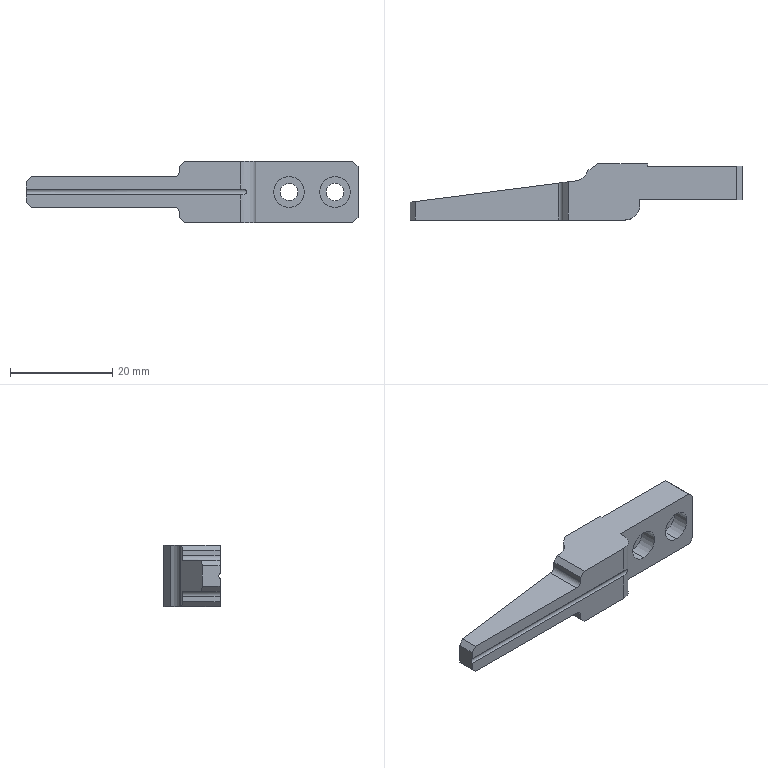Part | SolidWorks | features ICE 5, Chamfer 4, Fillet 2, Extrusion 1, HoleWzd 1 | 1 solid | 38 faces | box 65 x 11 x 12 mm | volume 4036 mm3 | plane 25 | cylinder 13 | commonest cylinder face diameters 6 x6 3.4 x4 2 x2 1.5 x1
STEP:
#1=CARTESIAN_POINT('',(28.,7.4,3.));
#2=VERTEX_POINT('',#1);
#3=CARTESIAN_POINT('',(28.,7.4,-3.));
#4=VERTEX_POINT('',#3);
#5=CARTESIAN_POINT('',(28.,7.4,0.));
#6=DIRECTION('',(0.,-1.,0.));
#7=DIRECTION('',(0.,0.,-1.));
#8=AXIS2_PLACEMENT_3D('',#5,#6,#7);
#9=CIRCLE('',#8,3.);
#10=EDGE_CURVE('',#2,#4,#9,.T.);
#11=ORIENTED_EDGE('',*,*,#10,.F.);
#12=CARTESIAN_POINT('',(28.,4.,3.));
#13=VERTEX_POINT('',#12);
#14=CARTESIAN_POINT('',(28.,4.,3.));
#15=DIRECTION('',(0.,-1.,0.));
#16=VECTOR('',#15,1000.);
#17=LINE('',#14,#16);
#18=EDGE_CURVE('',#2,#13,#17,.T.);
#19=ORIENTED_EDGE('',*,*,#18,.T.);
#20=CARTESIAN_POINT('',(28.,4.,-3.));
#21=VERTEX_POINT('',#20);
#22=CARTESIAN_POINT('',(28.,4.,0.));
#23=DIRECTION('',(0.,-1.,0.));
#24=DIRECTION('',(0.,0.,-1.));
#25=AXIS2_PLACEMENT_3D('',#22,#23,#24);
#26=CIRCLE('',#25,3.);
#27=EDGE_CURVE('',#13,#21,#26,.T.);
#28=ORIENTED_EDGE('',*,*,#27,.T.);
#29=CARTESIAN_POINT('',(28.,4.,-3.));
#30=DIRECTION('',(0.,-1.,0.));
#31=VECTOR('',#30,1000.);
#32=LINE('',#29,#31);
#33=EDGE_CURVE('',#4,#21,#32,.T.);
#34=ORIENTED_EDGE('',*,*,#33,.F.);
#35=EDGE_LOOP('',(#11,#19,#28,#34));
#36=FACE_OUTER_BOUND('',#35,.T.);
#37=CARTESIAN_POINT('',(28.,4.,0.));
#38=DIRECTION('',(0.,-1.,0.));
#39=DIRECTION('',(0.,0.,-1.));
#40=AXIS2_PLACEMENT_3D('',#37,#38,#39);
#41=CYLINDRICAL_SURFACE('',#40,3.);
#42=ADVANCED_FACE('',(#36),#41,.F.);
#43=CARTESIAN_POINT('',(19.,7.4,3.));
#44=VERTEX_POINT('',#43);
#45=CARTESIAN_POINT('',(19.,7.4,-3.));
#46=VERTEX_POINT('',#45);
#47=CARTESIAN_POINT('',(19.,7.4,0.));
#48=DIRECTION('',(0.,-1.,0.));
#49=DIRECTION('',(0.,0.,-1.));
#50=AXIS2_PLACEMENT_3D('',#47,#48,#49);
#51=CIRCLE('',#50,3.);
#52=EDGE_CURVE('',#44,#46,#51,.T.);
#53=ORIENTED_EDGE('',*,*,#52,.F.);
#54=CARTESIAN_POINT('',(19.,4.,3.));
#55=VERTEX_POINT('',#54);
#56=CARTESIAN_POINT('',(19.,4.,3.));
#57=DIRECTION('',(0.,-1.,0.));
#58=VECTOR('',#57,1000.);
#59=LINE('',#56,#58);
#60=EDGE_CURVE('',#44,#55,#59,.T.);
#61=ORIENTED_EDGE('',*,*,#60,.T.);
#62=CARTESIAN_POINT('',(19.,4.,-3.));
#63=VERTEX_POINT('',#62);
#64=CARTESIAN_POINT('',(19.,4.,0.));
#65=DIRECTION('',(0.,-1.,0.));
#66=DIRECTION('',(0.,0.,-1.));
#67=AXIS2_PLACEMENT_3D('',#64,#65,#66);
#68=CIRCLE('',#67,3.);
#69=EDGE_CURVE('',#55,#63,#68,.T.);
#70=ORIENTED_EDGE('',*,*,#69,.T.);
#71=CARTESIAN_POINT('',(19.,4.,-3.));
#72=DIRECTION('',(0.,-1.,0.));
#73=VECTOR('',#72,1000.);
#74=LINE('',#71,#73);
#75=EDGE_CURVE('',#46,#63,#74,.T.);
#76=ORIENTED_EDGE('',*,*,#75,.F.);
#77=EDGE_LOOP('',(#53,#61,#70,#76));
#78=FACE_OUTER_BOUND('',#77,.T.);
#79=CARTESIAN_POINT('',(19.,4.,0.));
#80=DIRECTION('',(0.,-1.,0.));
#81=DIRECTION('',(0.,0.,-1.));
#82=AXIS2_PLACEMENT_3D('',#79,#80,#81);
#83=CYLINDRICAL_SURFACE('',#82,3.);
#84=ADVANCED_FACE('',(#78),#83,.F.);
#85=CARTESIAN_POINT('',(28.,10.5,1.7));
#86=VERTEX_POINT('',#85);
#87=CARTESIAN_POINT('',(28.,10.5,-1.7));
#88=VERTEX_POINT('',#87);
#89=CARTESIAN_POINT('',(28.,10.5,0.));
#90=DIRECTION('',(0.,-1.,0.));
#91=DIRECTION('',(0.,0.,1.));
#92=AXIS2_PLACEMENT_3D('',#89,#90,#91);
#93=CIRCLE('',#92,1.7);
#94=EDGE_CURVE('',#86,#88,#93,.T.);
#95=ORIENTED_EDGE('',*,*,#94,.F.);
#96=CARTESIAN_POINT('',(28.,7.4,1.7));
#97=VERTEX_POINT('',#96);
#98=CARTESIAN_POINT('',(28.,4.,1.7));
#99=DIRECTION('',(0.,-1.,0.));
#100=VECTOR('',#99,1000.);
#101=LINE('',#98,#100);
#102=EDGE_CURVE('',#86,#97,#101,.T.);
#103=ORIENTED_EDGE('',*,*,#102,.T.);
#104=CARTESIAN_POINT('',(28.,7.4,-1.7));
#105=VERTEX_POINT('',#104);
#106=CARTESIAN_POINT('',(28.,7.4,0.));
#107=DIRECTION('',(0.,-1.,0.));
#108=DIRECTION('',(0.,0.,-1.));
#109=AXIS2_PLACEMENT_3D('',#106,#107,#108);
#110=CIRCLE('',#109,1.7);
#111=EDGE_CURVE('',#97,#105,#110,.T.);
#112=ORIENTED_EDGE('',*,*,#111,.T.);
#113=CARTESIAN_POINT('',(28.,4.,-1.7));
#114=DIRECTION('',(0.,-1.,0.));
#115=VECTOR('',#114,1000.);
#116=LINE('',#113,#115);
#117=EDGE_CURVE('',#88,#105,#116,.T.);
#118=ORIENTED_EDGE('',*,*,#117,.F.);
#119=EDGE_LOOP('',(#95,#103,#112,#118));
#120=FACE_OUTER_BOUND('',#119,.T.);
#121=CARTESIAN_POINT('',(28.,4.,0.));
#122=DIRECTION('',(0.,-1.,0.));
#123=DIRECTION('',(0.,0.,-1.));
#124=AXIS2_PLACEMENT_3D('',#121,#122,#123);
#125=CYLINDRICAL_SURFACE('',#124,1.7);
#126=ADVANCED_FACE('',(#120),#125,.F.);
#127=CARTESIAN_POINT('',(19.,10.5,1.7));
#128=VERTEX_POINT('',#127);
#129=CARTESIAN_POINT('',(19.,10.5,-1.7));
#130=VERTEX_POINT('',#129);
#131=CARTESIAN_POINT('',(19.,10.5,0.));
#132=DIRECTION('',(0.,-1.,0.));
#133=DIRECTION('',(0.,0.,1.));
#134=AXIS2_PLACEMENT_3D('',#131,#132,#133);
#135=CIRCLE('',#134,1.7);
#136=EDGE_CURVE('',#128,#130,#135,.T.);
#137=ORIENTED_EDGE('',*,*,#136,.F.);
#138=CARTESIAN_POINT('',(19.,7.4,1.7));
#139=VERTEX_POINT('',#138);
#140=CARTESIAN_POINT('',(19.,4.,1.7));
#141=DIRECTION('',(0.,-1.,0.));
#142=VECTOR('',#141,1000.);
#143=LINE('',#140,#142);
#144=EDGE_CURVE('',#128,#139,#143,.T.);
#145=ORIENTED_EDGE('',*,*,#144,.T.);
#146=CARTESIAN_POINT('',(19.,7.4,-1.7));
#147=VERTEX_POINT('',#146);
#148=CARTESIAN_POINT('',(19.,7.4,0.));
#149=DIRECTION('',(0.,-1.,0.));
#150=DIRECTION('',(0.,0.,-1.));
#151=AXIS2_PLACEMENT_3D('',#148,#149,#150);
#152=CIRCLE('',#151,1.7);
#153=EDGE_CURVE('',#139,#147,#152,.T.);
#154=ORIENTED_EDGE('',*,*,#153,.T.);
#155=CARTESIAN_POINT('',(19.,4.,-1.7));
#156=DIRECTION('',(0.,-1.,0.));
#157=VECTOR('',#156,1000.);
#158=LINE('',#155,#157);
#159=EDGE_CURVE('',#130,#147,#158,.T.);
#160=ORIENTED_EDGE('',*,*,#159,.F.);
#161=EDGE_LOOP('',(#137,#145,#154,#160));
#162=FACE_OUTER_BOUND('',#161,.T.);
#163=CARTESIAN_POINT('',(19.,4.,0.));
#164=DIRECTION('',(0.,-1.,0.));
#165=DIRECTION('',(0.,0.,-1.));
#166=AXIS2_PLACEMENT_3D('',#163,#164,#165);
#167=CYLINDRICAL_SURFACE('',#166,1.7);
#168=ADVANCED_FACE('',(#162),#167,.F.);
#169=CARTESIAN_POINT('',(32.5,10.5,5.));
#170=VERTEX_POINT('',#169);
#171=CARTESIAN_POINT('',(32.5,10.5,-5.));
#172=VERTEX_POINT('',#171);
#173=CARTESIAN_POINT('',(32.5,10.5,-6.));
#174=DIRECTION('',(0.,0.,-1.));
#175=VECTOR('',#174,1000.);
#176=LINE('',#173,#175);
#177=EDGE_CURVE('',#170,#172,#176,.T.);
#178=ORIENTED_EDGE('',*,*,#177,.F.);
#179=CARTESIAN_POINT('',(32.5,4.,5.));
#180=VERTEX_POINT('',#179);
#181=CARTESIAN_POINT('',(32.5,11.,5.));
#182=DIRECTION('',(0.,-1.,0.));
#183=VECTOR('',#182,1000.);
#184=LINE('',#181,#183);
#185=EDGE_CURVE('',#170,#180,#184,.T.);
#186=ORIENTED_EDGE('',*,*,#185,.T.);
#187=CARTESIAN_POINT('',(32.5,4.,-5.));
#188=VERTEX_POINT('',#187);
#189=CARTESIAN_POINT('',(32.5,4.,-14.));
#190=DIRECTION('',(0.,0.,1.));
#191=VECTOR('',#190,1000.);
#192=LINE('',#189,#191);
#193=EDGE_CURVE('',#188,#180,#192,.T.);
#194=ORIENTED_EDGE('',*,*,#193,.F.);
#195=CARTESIAN_POINT('',(32.5,11.,-5.));
#196=DIRECTION('',(0.,1.,0.));
#197=VECTOR('',#196,1000.);
#198=LINE('',#195,#197);
#199=EDGE_CURVE('',#188,#172,#198,.T.);
#200=ORIENTED_EDGE('',*,*,#199,.T.);
#201=EDGE_LOOP('',(#178,#186,#194,#200));
#202=FACE_OUTER_BOUND('',#201,.T.);
#203=CARTESIAN_POINT('',(32.5,11.,-6.));
#204=DIRECTION('',(-1.,0.,0.));
#205=DIRECTION('',(0.,0.,1.));
#206=AXIS2_PLACEMENT_3D('',#203,#204,#205);
#207=PLANE('',#206);
#208=ADVANCED_FACE('',(#202),#207,.F.);
#209=ORIENTED_EDGE('',*,*,#185,.F.);
#210=CARTESIAN_POINT('',(31.5,10.5,6.));
#211=VERTEX_POINT('',#210);
#212=CARTESIAN_POINT('',(32.5,10.5,5.));
#213=DIRECTION('',(-0.7071,0.,0.7071));
#214=VECTOR('',#213,1000.);
#215=LINE('',#212,#214);
#216=EDGE_CURVE('',#170,#211,#215,.T.);
#217=ORIENTED_EDGE('',*,*,#216,.T.);
#218=CARTESIAN_POINT('',(31.5,4.,6.));
#219=VERTEX_POINT('',#218);
#220=CARTESIAN_POINT('',(31.5,11.,6.));
#221=DIRECTION('',(0.,1.,0.));
#222=VECTOR('',#221,1000.);
#223=LINE('',#220,#222);
#224=EDGE_CURVE('',#219,#211,#223,.T.);
#225=ORIENTED_EDGE('',*,*,#224,.F.);
#226=CARTESIAN_POINT('',(32.5,4.,5.));
#227=DIRECTION('',(-0.7071,0.,0.7071));
#228=VECTOR('',#227,1000.);
#229=LINE('',#226,#228);
#230=EDGE_CURVE('',#180,#219,#229,.T.);
#231=ORIENTED_EDGE('',*,*,#230,.F.);
#232=EDGE_LOOP('',(#209,#217,#225,#231));
#233=FACE_OUTER_BOUND('',#232,.T.);
#234=CARTESIAN_POINT('',(32.5,11.,5.));
#235=DIRECTION('',(-0.7071,0.,-0.7071));
#236=DIRECTION('',(0.,-1.,0.));
#237=AXIS2_PLACEMENT_3D('',#234,#235,#236);
#238=PLANE('',#237);
#239=ADVANCED_FACE('',(#233),#238,.F.);
#240=CARTESIAN_POINT('',(31.5,10.5,-6.));
#241=VERTEX_POINT('',#240);
#242=CARTESIAN_POINT('',(31.5,4.,-6.));
#243=VERTEX_POINT('',#242);
#244=CARTESIAN_POINT('',(31.5,11.,-6.));
#245=DIRECTION('',(0.,-1.,0.));
#246=VECTOR('',#245,1000.);
#247=LINE('',#244,#246);
#248=EDGE_CURVE('',#241,#243,#247,.T.);
#249=ORIENTED_EDGE('',*,*,#248,.F.);
#250=CARTESIAN_POINT('',(31.5,10.5,-6.));
#251=DIRECTION('',(0.7071,0.,0.7071));
#252=VECTOR('',#251,1000.);
#253=LINE('',#250,#252);
#254=EDGE_CURVE('',#241,#172,#253,.T.);
#255=ORIENTED_EDGE('',*,*,#254,.T.);
#256=ORIENTED_EDGE('',*,*,#199,.F.);
#257=CARTESIAN_POINT('',(31.5,4.,-6.));
#258=DIRECTION('',(0.7071,0.,0.7071));
#259=VECTOR('',#258,1000.);
#260=LINE('',#257,#259);
#261=EDGE_CURVE('',#243,#188,#260,.T.);
#262=ORIENTED_EDGE('',*,*,#261,.F.);
#263=EDGE_LOOP('',(#249,#255,#256,#262));
#264=FACE_OUTER_BOUND('',#263,.T.);
#265=CARTESIAN_POINT('',(31.5,11.,-6.));
#266=DIRECTION('',(-0.7071,0.,0.7071));
#267=DIRECTION('',(0.,-1.,0.));
#268=AXIS2_PLACEMENT_3D('',#265,#266,#267);
#269=PLANE('',#268);
#270=ADVANCED_FACE('',(#264),#269,.F.);
#271=ORIENTED_EDGE('',*,*,#144,.F.);
#272=CARTESIAN_POINT('',(19.,10.5,0.));
#273=DIRECTION('',(0.,-1.,0.));
#274=DIRECTION('',(0.,0.,1.));
#275=AXIS2_PLACEMENT_3D('',#272,#273,#274);
#276=CIRCLE('',#275,1.7);
#277=EDGE_CURVE('',#130,#128,#276,.T.);
#278=ORIENTED_EDGE('',*,*,#277,.F.);
#279=ORIENTED_EDGE('',*,*,#159,.T.);
#280=CARTESIAN_POINT('',(19.,7.4,0.));
#281=DIRECTION('',(0.,-1.,0.));
#282=DIRECTION('',(0.,0.,-1.));
#283=AXIS2_PLACEMENT_3D('',#280,#281,#282);
#284=CIRCLE('',#283,1.7);
#285=EDGE_CURVE('',#147,#139,#284,.T.);
#286=ORIENTED_EDGE('',*,*,#285,.T.);
#287=EDGE_LOOP('',(#271,#278,#279,#286));
#288=FACE_OUTER_BOUND('',#287,.T.);
#289=CARTESIAN_POINT('',(19.,4.,0.));
#290=DIRECTION('',(0.,-1.,0.));
#291=DIRECTION('',(0.,0.,-1.));
#292=AXIS2_PLACEMENT_3D('',#289,#290,#291);
#293=CYLINDRICAL_SURFACE('',#292,1.7);
#294=ADVANCED_FACE('',(#288),#293,.F.);
#295=ORIENTED_EDGE('',*,*,#102,.F.);
#296=CARTESIAN_POINT('',(28.,10.5,0.));
#297=DIRECTION('',(0.,-1.,0.));
#298=DIRECTION('',(0.,0.,1.));
#299=AXIS2_PLACEMENT_3D('',#296,#297,#298);
#300=CIRCLE('',#299,1.7);
#301=EDGE_CURVE('',#88,#86,#300,.T.);
#302=ORIENTED_EDGE('',*,*,#301,.F.);
#303=ORIENTED_EDGE('',*,*,#117,.T.);
#304=CARTESIAN_POINT('',(28.,7.4,0.));
#305=DIRECTION('',(0.,-1.,0.));
#306=DIRECTION('',(0.,0.,-1.));
#307=AXIS2_PLACEMENT_3D('',#304,#305,#306);
#308=CIRCLE('',#307,1.7);
#309=EDGE_CURVE('',#105,#97,#308,.T.);
#310=ORIENTED_EDGE('',*,*,#309,.T.);
#311=EDGE_LOOP('',(#295,#302,#303,#310));
#312=FACE_OUTER_BOUND('',#311,.T.);
#313=CARTESIAN_POINT('',(28.,4.,0.));
#314=DIRECTION('',(0.,-1.,0.));
#315=DIRECTION('',(0.,0.,-1.));
#316=AXIS2_PLACEMENT_3D('',#313,#314,#315);
#317=CYLINDRICAL_SURFACE('',#316,1.7);
#318=ADVANCED_FACE('',(#312),#317,.F.);
#319=CARTESIAN_POINT('',(-2.5,0.,-5.));
#320=VERTEX_POINT('',#319);
#321=CARTESIAN_POINT('',(-2.5,0.,-4.));
#322=VERTEX_POINT('',#321);
#323=CARTESIAN_POINT('',(-2.5,0.,-6.));
#324=DIRECTION('',(0.,0.,1.));
#325=VECTOR('',#324,1000.);
#326=LINE('',#323,#325);
#327=EDGE_CURVE('',#320,#322,#326,.T.);
#328=ORIENTED_EDGE('',*,*,#327,.F.);
#329=CARTESIAN_POINT('',(-1.5,0.,-6.));
#330=VERTEX_POINT('',#329);
#331=CARTESIAN_POINT('',(-2.5,0.,-5.));
#332=DIRECTION('',(0.7071,0.,-0.7071));
#333=VECTOR('',#332,1000.);
#334=LINE('',#331,#333);
#335=EDGE_CURVE('',#320,#330,#334,.T.);
#336=ORIENTED_EDGE('',*,*,#335,.T.);
#337=CARTESIAN_POINT('',(9.5,0.,-6.));
#338=VERTEX_POINT('',#337);
#339=CARTESIAN_POINT('',(-32.5,0.,-6.));
#340=DIRECTION('',(-1.,0.,0.));
#341=VECTOR('',#340,1000.);
#342=LINE('',#339,#341);
#343=EDGE_CURVE('',#338,#330,#342,.T.);
#344=ORIENTED_EDGE('',*,*,#343,.F.);
#345=CARTESIAN_POINT('',(9.5,0.,-0.559));
#346=VERTEX_POINT('',#345);
#347=CARTESIAN_POINT('',(9.5,0.,0.));
#348=DIRECTION('',(0.,0.,1.));
#349=VECTOR('',#348,1000.);
#350=LINE('',#347,#349);
#351=EDGE_CURVE('',#338,#346,#350,.T.);
#352=ORIENTED_EDGE('',*,*,#351,.T.);
#353=CARTESIAN_POINT('',(-32.5,0.,-0.559));
#354=VERTEX_POINT('',#353);
#355=CARTESIAN_POINT('',(32.5,0.,-0.559));
#356=DIRECTION('',(-1.,0.,0.));
#357=VECTOR('',#356,1000.);
#358=LINE('',#355,#357);
#359=EDGE_CURVE('',#346,#354,#358,.T.);
#360=ORIENTED_EDGE('',*,*,#359,.T.);
#361=CARTESIAN_POINT('',(-32.5,0.,-2.));
#362=VERTEX_POINT('',#361);
#363=CARTESIAN_POINT('',(-32.5,0.,-6.));
#364=DIRECTION('',(0.,0.,1.));
#365=VECTOR('',#364,1000.);
#366=LINE('',#363,#365);
#367=EDGE_CURVE('',#362,#354,#366,.T.);
#368=ORIENTED_EDGE('',*,*,#367,.F.);
#369=CARTESIAN_POINT('',(-31.5,0.,-3.));
#370=VERTEX_POINT('',#369);
#371=CARTESIAN_POINT('',(-32.5,0.,-2.));
#372=DIRECTION('',(0.7071,0.,-0.7071));
#373=VECTOR('',#372,1000.);
#374=LINE('',#371,#373);
#375=EDGE_CURVE('',#362,#370,#374,.T.);
#376=ORIENTED_EDGE('',*,*,#375,.T.);
#377=CARTESIAN_POINT('',(-3.5,0.,-3.));
#378=VERTEX_POINT('',#377);
#379=CARTESIAN_POINT('',(-32.5,0.,-3.));
#380=DIRECTION('',(-1.,0.,0.));
#381=VECTOR('',#380,1000.);
#382=LINE('',#379,#381);
#383=EDGE_CURVE('',#378,#370,#382,.T.);
#384=ORIENTED_EDGE('',*,*,#383,.F.);
#385=CARTESIAN_POINT('',(-3.5,0.,-4.));
#386=DIRECTION('',(0.,1.,0.));
#387=DIRECTION('',(0.,0.,1.));
#388=AXIS2_PLACEMENT_3D('',#385,#386,#387);
#389=CIRCLE('',#388,1.);
#390=EDGE_CURVE('',#378,#322,#389,.T.);
#391=ORIENTED_EDGE('',*,*,#390,.T.);
#392=EDGE_LOOP('',(#328,#336,#344,#352,#360,#368,#376,#384,#391));
#393=FACE_OUTER_BOUND('',#392,.T.);
#394=CARTESIAN_POINT('',(0.,0.,0.));
#395=DIRECTION('',(0.,1.,0.));
#396=DIRECTION('',(0.,0.,1.));
#397=AXIS2_PLACEMENT_3D('',#394,#395,#396);
#398=PLANE('',#397);
#399=ADVANCED_FACE('',(#393),#398,.F.);
#400=CARTESIAN_POINT('',(14.,11.,-6.));
#401=VERTEX_POINT('',#400);
#402=CARTESIAN_POINT('',(4.224,11.,-6.));
#403=VERTEX_POINT('',#402);
#404=CARTESIAN_POINT('',(-32.5,11.,-6.));
#405=DIRECTION('',(-1.,0.,0.));
#406=VECTOR('',#405,1000.);
#407=LINE('',#404,#406);
#408=EDGE_CURVE('',#401,#403,#407,.T.);
#409=ORIENTED_EDGE('',*,*,#408,.F.);
#410=CARTESIAN_POINT('',(14.,10.5,-6.));
#411=VERTEX_POINT('',#410);
#412=CARTESIAN_POINT('',(14.,10.5,-6.));
#413=DIRECTION('',(0.,1.,0.));
#414=VECTOR('',#413,1000.);
#415=LINE('',#412,#414);
#416=EDGE_CURVE('',#411,#401,#415,.T.);
#417=ORIENTED_EDGE('',*,*,#416,.F.);
#418=CARTESIAN_POINT('',(14.,10.5,-6.));
#419=DIRECTION('',(-1.,0.,0.));
#420=VECTOR('',#419,1000.);
#421=LINE('',#418,#420);
#422=EDGE_CURVE('',#241,#411,#421,.T.);
#423=ORIENTED_EDGE('',*,*,#422,.F.);
#424=ORIENTED_EDGE('',*,*,#248,.T.);
#425=CARTESIAN_POINT('',(12.5,4.,-6.));
#426=VERTEX_POINT('',#425);
#427=CARTESIAN_POINT('',(-32.5,4.,-6.));
#428=DIRECTION('',(-1.,0.,0.));
#429=VECTOR('',#428,1000.);
#430=LINE('',#427,#429);
#431=EDGE_CURVE('',#243,#426,#430,.T.);
#432=ORIENTED_EDGE('',*,*,#431,.T.);
#433=CARTESIAN_POINT('',(12.5,3.,-6.));
#434=VERTEX_POINT('',#433);
#435=CARTESIAN_POINT('',(12.5,11.,-6.));
#436=DIRECTION('',(0.,-1.,0.));
#437=VECTOR('',#436,1000.);
#438=LINE('',#435,#437);
#439=EDGE_CURVE('',#426,#434,#438,.T.);
#440=ORIENTED_EDGE('',*,*,#439,.T.);
#441=CARTESIAN_POINT('',(9.5,3.,-6.));
#442=DIRECTION('',(0.,0.,-1.));
#443=DIRECTION('',(1.,0.,0.));
#444=AXIS2_PLACEMENT_3D('',#441,#442,#443);
#445=CIRCLE('',#444,3.);
#446=EDGE_CURVE('',#434,#338,#445,.T.);
#447=ORIENTED_EDGE('',*,*,#446,.T.);
#448=ORIENTED_EDGE('',*,*,#343,.T.);
#449=CARTESIAN_POINT('',(-1.5,7.486,-6.));
#450=VERTEX_POINT('',#449);
#451=CARTESIAN_POINT('',(-1.5,11.,-6.));
#452=DIRECTION('',(0.,1.,0.));
#453=VECTOR('',#452,1000.);
#454=LINE('',#451,#453);
#455=EDGE_CURVE('',#330,#450,#454,.T.);
#456=ORIENTED_EDGE('',*,*,#455,.T.);
#457=CARTESIAN_POINT('',(-0.1174,7.663,-6.));
#458=VERTEX_POINT('',#457);
#459=CARTESIAN_POINT('',(-31.551,3.622,-6.));
#460=DIRECTION('',(0.9918,0.1275,0.));
#461=VECTOR('',#460,1000.);
#462=LINE('',#459,#461);
#463=EDGE_CURVE('',#450,#458,#462,.T.);
#464=ORIENTED_EDGE('',*,*,#463,.T.);
#465=CARTESIAN_POINT('',(2.334,9.656,-6.));
#466=VERTEX_POINT('',#465);
#467=CARTESIAN_POINT('',(-0.5,10.639,-6.));
#468=DIRECTION('',(0.,0.,1.));
#469=DIRECTION('',(1.,0.,0.));
#470=AXIS2_PLACEMENT_3D('',#467,#468,#469);
#471=CIRCLE('',#470,3.);
#472=EDGE_CURVE('',#458,#466,#471,.T.);
#473=ORIENTED_EDGE('',*,*,#472,.T.);
#474=CARTESIAN_POINT('',(2.334,9.656,-6.));
#475=DIRECTION('',(0.8148,0.5797,0.));
#476=VECTOR('',#475,1000.);
#477=LINE('',#474,#476);
#478=EDGE_CURVE('',#466,#403,#477,.T.);
#479=ORIENTED_EDGE('',*,*,#478,.T.);
#480=EDGE_LOOP('',(#409,#417,#423,#424,#432,#440,#447,#448,#456,#464,#473,#479));
#481=FACE_OUTER_BOUND('',#480,.T.);
#482=CARTESIAN_POINT('',(-32.5,11.,-6.));
#483=DIRECTION('',(0.,0.,1.));
#484=DIRECTION('',(1.,0.,0.));
#485=AXIS2_PLACEMENT_3D('',#482,#483,#484);
#486=PLANE('',#485);
#487=ADVANCED_FACE('',(#481),#486,.F.);
#488=CARTESIAN_POINT('',(-32.5,3.5,-2.));
#489=VERTEX_POINT('',#488);
#490=CARTESIAN_POINT('',(-32.5,3.5,2.));
#491=VERTEX_POINT('',#490);
#492=CARTESIAN_POINT('',(-32.5,3.5,-14.));
#493=DIRECTION('',(0.,0.,1.));
#494=VECTOR('',#493,1000.);
#495=LINE('',#492,#494);
#496=EDGE_CURVE('',#489,#491,#495,.T.);
#497=ORIENTED_EDGE('',*,*,#496,.F.);
#498=CARTESIAN_POINT('',(-32.5,11.,-2.));
#499=DIRECTION('',(0.,-1.,0.));
#500=VECTOR('',#499,1000.);
#501=LINE('',#498,#500);
#502=EDGE_CURVE('',#489,#362,#501,.T.);
#503=ORIENTED_EDGE('',*,*,#502,.T.);
#504=ORIENTED_EDGE('',*,*,#367,.T.);
#505=CARTESIAN_POINT('',(-32.5,0.,0.559));
#506=VERTEX_POINT('',#505);
#507=CARTESIAN_POINT('',(-32.5,-0.5,0.));
#508=DIRECTION('',(-1.,0.,0.));
#509=DIRECTION('',(0.,0.,1.));
#510=AXIS2_PLACEMENT_3D('',#507,#508,#509);
#511=CIRCLE('',#510,0.75);
#512=EDGE_CURVE('',#506,#354,#511,.T.);
#513=ORIENTED_EDGE('',*,*,#512,.F.);
#514=CARTESIAN_POINT('',(-32.5,0.,2.));
#515=VERTEX_POINT('',#514);
#516=CARTESIAN_POINT('',(-32.5,0.,-6.));
#517=DIRECTION('',(0.,0.,1.));
#518=VECTOR('',#517,1000.);
#519=LINE('',#516,#518);
#520=EDGE_CURVE('',#506,#515,#519,.T.);
#521=ORIENTED_EDGE('',*,*,#520,.T.);
#522=CARTESIAN_POINT('',(-32.5,11.,2.));
#523=DIRECTION('',(0.,1.,0.));
#524=VECTOR('',#523,1000.);
#525=LINE('',#522,#524);
#526=EDGE_CURVE('',#515,#491,#525,.T.);
#527=ORIENTED_EDGE('',*,*,#526,.T.);
#528=EDGE_LOOP('',(#497,#503,#504,#513,#521,#527));
#529=FACE_OUTER_BOUND('',#528,.T.);
#530=CARTESIAN_POINT('',(-32.5,11.,-6.));
#531=DIRECTION('',(1.,0.,0.));
#532=DIRECTION('',(0.,0.,-1.));
#533=AXIS2_PLACEMENT_3D('',#530,#531,#532);
#534=PLANE('',#533);
#535=ADVANCED_FACE('',(#529),#534,.F.);
#536=CARTESIAN_POINT('',(14.,10.5,6.));
#537=VERTEX_POINT('',#536);
#538=CARTESIAN_POINT('',(14.,10.5,6.));
#539=DIRECTION('',(1.,0.,0.));
#540=VECTOR('',#539,1000.);
#541=LINE('',#538,#540);
#542=EDGE_CURVE('',#537,#211,#541,.T.);
#543=ORIENTED_EDGE('',*,*,#542,.F.);
#544=CARTESIAN_POINT('',(14.,11.,6.));
#545=VERTEX_POINT('',#544);
#546=CARTESIAN_POINT('',(14.,10.5,6.));
#547=DIRECTION('',(0.,1.,0.));
#548=VECTOR('',#547,1000.);
#549=LINE('',#546,#548);
#550=EDGE_CURVE('',#537,#545,#549,.T.);
#551=ORIENTED_EDGE('',*,*,#550,.T.);
#552=CARTESIAN_POINT('',(4.224,11.,6.));
#553=VERTEX_POINT('',#552);
#554=CARTESIAN_POINT('',(-32.5,11.,6.));
#555=DIRECTION('',(1.,0.,0.));
#556=VECTOR('',#555,1000.);
#557=LINE('',#554,#556);
#558=EDGE_CURVE('',#553,#545,#557,.T.);
#559=ORIENTED_EDGE('',*,*,#558,.F.);
#560=CARTESIAN_POINT('',(2.334,9.656,6.));
#561=VERTEX_POINT('',#560);
#562=CARTESIAN_POINT('',(2.334,9.656,6.));
#563=DIRECTION('',(-0.8148,-0.5797,0.));
#564=VECTOR('',#563,1000.);
#565=LINE('',#562,#564);
#566=EDGE_CURVE('',#553,#561,#565,.T.);
#567=ORIENTED_EDGE('',*,*,#566,.T.);
#568=CARTESIAN_POINT('',(-0.1174,7.663,6.));
#569=VERTEX_POINT('',#568);
#570=CARTESIAN_POINT('',(-0.5,10.639,6.));
#571=DIRECTION('',(0.,0.,-1.));
#572=DIRECTION('',(-1.,0.,0.));
#573=AXIS2_PLACEMENT_3D('',#570,#571,#572);
#574=CIRCLE('',#573,3.);
#575=EDGE_CURVE('',#561,#569,#574,.T.);
#576=ORIENTED_EDGE('',*,*,#575,.T.);
#577=CARTESIAN_POINT('',(-1.5,7.486,6.));
#578=VERTEX_POINT('',#577);
#579=CARTESIAN_POINT('',(-32.5,3.5,6.));
#580=DIRECTION('',(0.9918,0.1275,0.));
#581=VECTOR('',#580,1000.);
#582=LINE('',#579,#581);
#583=EDGE_CURVE('',#578,#569,#582,.T.);
#584=ORIENTED_EDGE('',*,*,#583,.F.);
#585=CARTESIAN_POINT('',(-1.5,0.,6.));
#586=VERTEX_POINT('',#585);
#587=CARTESIAN_POINT('',(-1.5,11.,6.));
#588=DIRECTION('',(0.,-1.,0.));
#589=VECTOR('',#588,1000.);
#590=LINE('',#587,#589);
#591=EDGE_CURVE('',#578,#586,#590,.T.);
#592=ORIENTED_EDGE('',*,*,#591,.T.);
#593=CARTESIAN_POINT('',(9.5,0.,6.));
#594=VERTEX_POINT('',#593);
#595=CARTESIAN_POINT('',(-32.5,0.,6.));
#596=DIRECTION('',(1.,0.,0.));
#597=VECTOR('',#596,1000.);
#598=LINE('',#595,#597);
#599=EDGE_CURVE('',#586,#594,#598,.T.);
#600=ORIENTED_EDGE('',*,*,#599,.T.);
#601=CARTESIAN_POINT('',(12.5,3.,6.));
#602=VERTEX_POINT('',#601);
#603=CARTESIAN_POINT('',(9.5,3.,6.));
#604=DIRECTION('',(0.,0.,1.));
#605=DIRECTION('',(-1.,0.,0.));
#606=AXIS2_PLACEMENT_3D('',#603,#604,#605);
#607=CIRCLE('',#606,3.);
#608=EDGE_CURVE('',#594,#602,#607,.T.);
#609=ORIENTED_EDGE('',*,*,#608,.T.);
#610=CARTESIAN_POINT('',(12.5,4.,6.));
#611=VERTEX_POINT('',#610);
#612=CARTESIAN_POINT('',(12.5,0.,6.));
#613=DIRECTION('',(0.,-1.,0.));
#614=VECTOR('',#613,1000.);
#615=LINE('',#612,#614);
#616=EDGE_CURVE('',#611,#602,#615,.T.);
#617=ORIENTED_EDGE('',*,*,#616,.F.);
#618=CARTESIAN_POINT('',(32.5,4.,6.));
#619=DIRECTION('',(-1.,0.,0.));
#620=VECTOR('',#619,1000.);
#621=LINE('',#618,#620);
#622=EDGE_CURVE('',#219,#611,#621,.T.);
#623=ORIENTED_EDGE('',*,*,#622,.F.);
#624=ORIENTED_EDGE('',*,*,#224,.T.);
#625=EDGE_LOOP('',(#543,#551,#559,#567,#576,#584,#592,#600,#609,#617,#623,#624));
#626=FACE_OUTER_BOUND('',#625,.T.);
#627=CARTESIAN_POINT('',(-32.5,11.,6.));
#628=DIRECTION('',(0.,0.,-1.));
#629=DIRECTION('',(-1.,0.,0.));
#630=AXIS2_PLACEMENT_3D('',#627,#628,#629);
#631=PLANE('',#630);
#632=ADVANCED_FACE('',(#626),#631,.F.);
#633=CARTESIAN_POINT('',(14.,11.,-6.));
#634=DIRECTION('',(0.,0.,1.));
#635=VECTOR('',#634,1000.);
#636=LINE('',#633,#635);
#637=EDGE_CURVE('',#401,#545,#636,.T.);
#638=ORIENTED_EDGE('',*,*,#637,.F.);
#639=ORIENTED_EDGE('',*,*,#408,.T.);
#640=CARTESIAN_POINT('',(4.224,11.,6.));
#641=DIRECTION('',(0.,0.,1.));
#642=VECTOR('',#641,1000.);
#643=LINE('',#640,#642);
#644=EDGE_CURVE('',#403,#553,#643,.T.);
#645=ORIENTED_EDGE('',*,*,#644,.T.);
#646=ORIENTED_EDGE('',*,*,#558,.T.);
#647=EDGE_LOOP('',(#638,#639,#645,#646));
#648=FACE_OUTER_BOUND('',#647,.T.);
#649=CARTESIAN_POINT('',(0.,11.,0.));
#650=DIRECTION('',(0.,1.,0.));
#651=DIRECTION('',(0.,0.,1.));
#652=AXIS2_PLACEMENT_3D('',#649,#650,#651);
#653=PLANE('',#652);
#654=ADVANCED_FACE('',(#648),#653,.T.);
#655=ORIENTED_EDGE('',*,*,#599,.F.);
#656=CARTESIAN_POINT('',(-2.5,0.,5.));
#657=VERTEX_POINT('',#656);
#658=CARTESIAN_POINT('',(-1.5,0.,6.));
#659=DIRECTION('',(-0.7071,0.,-0.7071));
#660=VECTOR('',#659,1000.);
#661=LINE('',#658,#660);
#662=EDGE_CURVE('',#586,#657,#661,.T.);
#663=ORIENTED_EDGE('',*,*,#662,.T.);
#664=CARTESIAN_POINT('',(-2.5,0.,4.));
#665=VERTEX_POINT('',#664);
#666=CARTESIAN_POINT('',(-2.5,0.,6.));
#667=DIRECTION('',(0.,0.,1.));
#668=VECTOR('',#667,1000.);
#669=LINE('',#666,#668);
#670=EDGE_CURVE('',#665,#657,#669,.T.);
#671=ORIENTED_EDGE('',*,*,#670,.F.);
#672=CARTESIAN_POINT('',(-3.5,0.,3.));
#673=VERTEX_POINT('',#672);
#674=CARTESIAN_POINT('',(-3.5,0.,4.));
#675=DIRECTION('',(0.,1.,0.));
#676=DIRECTION('',(0.,0.,1.));
#677=AXIS2_PLACEMENT_3D('',#674,#675,#676);
#678=CIRCLE('',#677,1.);
#679=EDGE_CURVE('',#665,#673,#678,.T.);
#680=ORIENTED_EDGE('',*,*,#679,.T.);
#681=CARTESIAN_POINT('',(-31.5,0.,3.));
#682=VERTEX_POINT('',#681);
#683=CARTESIAN_POINT('',(-32.5,0.,3.));
#684=DIRECTION('',(1.,0.,0.));
#685=VECTOR('',#684,1000.);
#686=LINE('',#683,#685);
#687=EDGE_CURVE('',#682,#673,#686,.T.);
#688=ORIENTED_EDGE('',*,*,#687,.F.);
#689=CARTESIAN_POINT('',(-31.5,0.,3.));
#690=DIRECTION('',(-0.7071,0.,-0.7071));
#691=VECTOR('',#690,1000.);
#692=LINE('',#689,#691);
#693=EDGE_CURVE('',#682,#515,#692,.T.);
#694=ORIENTED_EDGE('',*,*,#693,.T.);
#695=ORIENTED_EDGE('',*,*,#520,.F.);
#696=CARTESIAN_POINT('',(9.5,0.,0.559));
#697=VERTEX_POINT('',#696);
#698=CARTESIAN_POINT('',(32.5,0.,0.559));
#699=DIRECTION('',(1.,0.,0.));
#700=VECTOR('',#699,1000.);
#701=LINE('',#698,#700);
#702=EDGE_CURVE('',#506,#697,#701,.T.);
#703=ORIENTED_EDGE('',*,*,#702,.T.);
#704=CARTESIAN_POINT('',(9.5,0.,0.));
#705=DIRECTION('',(0.,0.,1.));
#706=VECTOR('',#705,1000.);
#707=LINE('',#704,#706);
#708=EDGE_CURVE('',#697,#594,#707,.T.);
#709=ORIENTED_EDGE('',*,*,#708,.T.);
#710=EDGE_LOOP('',(#655,#663,#671,#680,#688,#694,#695,#703,#709));
#711=FACE_OUTER_BOUND('',#710,.T.);
#712=CARTESIAN_POINT('',(0.,0.,0.));
#713=DIRECTION('',(0.,1.,0.));
#714=DIRECTION('',(0.,0.,1.));
#715=AXIS2_PLACEMENT_3D('',#712,#713,#714);
#716=PLANE('',#715);
#717=ADVANCED_FACE('',(#711),#716,.F.);
#718=CARTESIAN_POINT('',(28.,4.,0.));
#719=DIRECTION('',(0.,-1.,0.));
#720=DIRECTION('',(0.,0.,-1.));
#721=AXIS2_PLACEMENT_3D('',#718,#719,#720);
#722=CIRCLE('',#721,3.);
#723=EDGE_CURVE('',#21,#13,#722,.T.);
#724=ORIENTED_EDGE('',*,*,#723,.F.);
#725=ORIENTED_EDGE('',*,*,#27,.F.);
#726=EDGE_LOOP('',(#724,#725));
#727=FACE_BOUND('',#726,.T.);
#728=CARTESIAN_POINT('',(19.,4.,0.));
#729=DIRECTION('',(0.,-1.,0.));
#730=DIRECTION('',(0.,0.,-1.));
#731=AXIS2_PLACEMENT_3D('',#728,#729,#730);
#732=CIRCLE('',#731,3.);
#733=EDGE_CURVE('',#63,#55,#732,.T.);
#734=ORIENTED_EDGE('',*,*,#733,.F.);
#735=ORIENTED_EDGE('',*,*,#69,.F.);
#736=EDGE_LOOP('',(#734,#735));
#737=FACE_BOUND('',#736,.T.);
#738=ORIENTED_EDGE('',*,*,#193,.T.);
#739=ORIENTED_EDGE('',*,*,#230,.T.);
#740=ORIENTED_EDGE('',*,*,#622,.T.);
#741=CARTESIAN_POINT('',(12.5,4.,-14.));
#742=DIRECTION('',(0.,0.,1.));
#743=VECTOR('',#742,1000.);
#744=LINE('',#741,#743);
#745=EDGE_CURVE('',#426,#611,#744,.T.);
#746=ORIENTED_EDGE('',*,*,#745,.F.);
#747=ORIENTED_EDGE('',*,*,#431,.F.);
#748=ORIENTED_EDGE('',*,*,#261,.T.);
#749=EDGE_LOOP('',(#738,#739,#740,#746,#747,#748));
#750=FACE_OUTER_BOUND('',#749,.T.);
#751=CARTESIAN_POINT('',(32.5,4.,-14.));
#752=DIRECTION('',(0.,1.,0.));
#753=DIRECTION('',(-1.,0.,0.));
#754=AXIS2_PLACEMENT_3D('',#751,#752,#753);
#755=PLANE('',#754);
#756=ADVANCED_FACE('',(#727,#737,#750),#755,.F.);
#757=ORIENTED_EDGE('',*,*,#616,.T.);
#758=CARTESIAN_POINT('',(12.5,3.,-14.));
#759=DIRECTION('',(0.,0.,-1.));
#760=VECTOR('',#759,1000.);
#761=LINE('',#758,#760);
#762=EDGE_CURVE('',#602,#434,#761,.T.);
#763=ORIENTED_EDGE('',*,*,#762,.T.);
#764=ORIENTED_EDGE('',*,*,#439,.F.);
#765=ORIENTED_EDGE('',*,*,#745,.T.);
#766=EDGE_LOOP('',(#757,#763,#764,#765));
#767=FACE_OUTER_BOUND('',#766,.T.);
#768=CARTESIAN_POINT('',(12.5,0.,-14.));
#769=DIRECTION('',(-1.,0.,0.));
#770=DIRECTION('',(0.,0.,1.));
#771=AXIS2_PLACEMENT_3D('',#768,#769,#770);
#772=PLANE('',#771);
#773=ADVANCED_FACE('',(#767),#772,.F.);
#774=ORIENTED_EDGE('',*,*,#463,.F.);
#775=CARTESIAN_POINT('',(-2.5,7.357,-5.));
#776=VERTEX_POINT('',#775);
#777=CARTESIAN_POINT('',(-2.268,7.387,-5.232));
#778=DIRECTION('',(-0.7042,-0.09054,0.7042));
#779=VECTOR('',#778,1000.);
#780=LINE('',#777,#779);
#781=EDGE_CURVE('',#450,#776,#780,.T.);
#782=ORIENTED_EDGE('',*,*,#781,.T.);
#783=CARTESIAN_POINT('',(-2.5,7.357,-4.));
#784=VERTEX_POINT('',#783);
#785=CARTESIAN_POINT('',(-2.5,7.357,-14.));
#786=DIRECTION('',(0.,0.,1.));
#787=VECTOR('',#786,1000.);
#788=LINE('',#785,#787);
#789=EDGE_CURVE('',#776,#784,#788,.T.);
#790=ORIENTED_EDGE('',*,*,#789,.T.);
#791=CARTESIAN_POINT('',(-3.5,7.229,-3.));
#792=VERTEX_POINT('',#791);
#793=CARTESIAN_POINT('',(-2.5,7.357,-4.));
#794=CARTESIAN_POINT('',(-2.5,7.357,-3.414));
#795=CARTESIAN_POINT('',(-2.914,7.304,-3.));
#796=CARTESIAN_POINT('',(-3.5,7.229,-3.));
#797=(BOUNDED_CURVE()B_SPLINE_CURVE(3,(#793,#794,#795,#796),.UNSPECIFIED.,.F.,.T.)B_SPLINE_CURVE_WITH_KNOTS((4,4),(0.,1.571),.UNSPECIFIED.)CURVE()GEOMETRIC_REPRESENTATION_ITEM()RATIONAL_B_SPLINE_CURVE((1.,0.8047,0.8047,1.))REPRESENTATION_ITEM(''));
#798=EDGE_CURVE('',#784,#792,#797,.T.);
#799=ORIENTED_EDGE('',*,*,#798,.T.);
#800=CARTESIAN_POINT('',(-31.5,3.629,-3.));
#801=VERTEX_POINT('',#800);
#802=CARTESIAN_POINT('',(-32.5,3.5,-3.));
#803=DIRECTION('',(-0.9918,-0.1275,0.));
#804=VECTOR('',#803,1000.);
#805=LINE('',#802,#804);
#806=EDGE_CURVE('',#792,#801,#805,.T.);
#807=ORIENTED_EDGE('',*,*,#806,.T.);
#808=CARTESIAN_POINT('',(-32.022,3.561,-2.478));
#809=DIRECTION('',(-0.7042,-0.09054,0.7042));
#810=VECTOR('',#809,1000.);
#811=LINE('',#808,#810);
#812=EDGE_CURVE('',#801,#489,#811,.T.);
#813=ORIENTED_EDGE('',*,*,#812,.T.);
#814=ORIENTED_EDGE('',*,*,#496,.T.);
#815=CARTESIAN_POINT('',(-31.5,3.629,3.));
#816=VERTEX_POINT('',#815);
#817=CARTESIAN_POINT('',(-31.03,3.689,3.47));
#818=DIRECTION('',(0.7042,0.09054,0.7042));
#819=VECTOR('',#818,1000.);
#820=LINE('',#817,#819);
#821=EDGE_CURVE('',#491,#816,#820,.T.);
#822=ORIENTED_EDGE('',*,*,#821,.T.);
#823=CARTESIAN_POINT('',(-3.5,7.229,3.));
#824=VERTEX_POINT('',#823);
#825=CARTESIAN_POINT('',(-32.5,3.5,3.));
#826=DIRECTION('',(0.9918,0.1275,0.));
#827=VECTOR('',#826,1000.);
#828=LINE('',#825,#827);
#829=EDGE_CURVE('',#816,#824,#828,.T.);
#830=ORIENTED_EDGE('',*,*,#829,.T.);
#831=CARTESIAN_POINT('',(-2.5,7.357,4.));
#832=VERTEX_POINT('',#831);
#833=CARTESIAN_POINT('',(-3.5,7.229,3.));
#834=CARTESIAN_POINT('',(-2.914,7.304,3.));
#835=CARTESIAN_POINT('',(-2.5,7.357,3.414));
#836=CARTESIAN_POINT('',(-2.5,7.357,4.));
#837=(BOUNDED_CURVE()B_SPLINE_CURVE(3,(#833,#834,#835,#836),.UNSPECIFIED.,.F.,.T.)B_SPLINE_CURVE_WITH_KNOTS((4,4),(4.712,6.283),.UNSPECIFIED.)CURVE()GEOMETRIC_REPRESENTATION_ITEM()RATIONAL_B_SPLINE_CURVE((1.,0.8047,0.8047,1.))REPRESENTATION_ITEM(''));
#838=EDGE_CURVE('',#824,#832,#837,.T.);
#839=ORIENTED_EDGE('',*,*,#838,.T.);
#840=CARTESIAN_POINT('',(-2.5,7.357,5.));
#841=VERTEX_POINT('',#840);
#842=CARTESIAN_POINT('',(-2.5,7.357,-14.));
#843=DIRECTION('',(0.,0.,1.));
#844=VECTOR('',#843,1000.);
#845=LINE('',#842,#844);
#846=EDGE_CURVE('',#832,#841,#845,.T.);
#847=ORIENTED_EDGE('',*,*,#846,.T.);
#848=CARTESIAN_POINT('',(-1.276,7.515,6.224));
#849=DIRECTION('',(0.7042,0.09054,0.7042));
#850=VECTOR('',#849,1000.);
#851=LINE('',#848,#850);
#852=EDGE_CURVE('',#841,#578,#851,.T.);
#853=ORIENTED_EDGE('',*,*,#852,.T.);
#854=ORIENTED_EDGE('',*,*,#583,.T.);
#855=CARTESIAN_POINT('',(-0.1174,7.663,-6.));
#856=DIRECTION('',(0.,0.,-1.));
#857=VECTOR('',#856,1000.);
#858=LINE('',#855,#857);
#859=EDGE_CURVE('',#569,#458,#858,.T.);
#860=ORIENTED_EDGE('',*,*,#859,.T.);
#861=EDGE_LOOP('',(#774,#782,#790,#799,#807,#813,#814,#822,#830,#839,#847,#853,#854,#860));
#862=FACE_OUTER_BOUND('',#861,.T.);
#863=CARTESIAN_POINT('',(-32.5,3.5,-14.));
#864=DIRECTION('',(0.1275,-0.9918,0.));
#865=DIRECTION('',(0.9918,0.1275,0.));
#866=AXIS2_PLACEMENT_3D('',#863,#864,#865);
#867=PLANE('',#866);
#868=ADVANCED_FACE('',(#862),#867,.F.);
#869=CARTESIAN_POINT('',(9.5,0.,-0.559));
#870=CARTESIAN_POINT('',(9.623,0.,-0.559));
#871=CARTESIAN_POINT('',(9.744,0.007495,-0.5526));
#872=CARTESIAN_POINT('',(9.982,0.03649,-0.5245));
#873=CARTESIAN_POINT('',(10.099,0.05802,-0.5031));
#874=CARTESIAN_POINT('',(10.328,0.1142,-0.4327));
#875=CARTESIAN_POINT('',(10.438,0.1486,-0.3854));
#876=CARTESIAN_POINT('',(10.576,0.1993,-0.2741));
#877=CARTESIAN_POINT('',(10.618,0.2159,-0.2298));
#878=CARTESIAN_POINT('',(10.679,0.2411,-0.1268));
#879=CARTESIAN_POINT('',(10.698,0.2496,-0.06647));
#880=CARTESIAN_POINT('',(10.7,0.2503,0.05807));
#881=CARTESIAN_POINT('',(10.682,0.2425,0.1191));
#882=CARTESIAN_POINT('',(10.622,0.2176,0.2247));
#883=CARTESIAN_POINT('',(10.581,0.2013,0.2691));
#884=CARTESIAN_POINT('',(10.443,0.1505,0.3824));
#885=CARTESIAN_POINT('',(10.334,0.1157,0.4306));
#886=CARTESIAN_POINT('',(10.105,0.05938,0.5016));
#887=CARTESIAN_POINT('',(9.988,0.03739,0.5236));
#888=CARTESIAN_POINT('',(9.746,0.007651,0.5525));
#889=CARTESIAN_POINT('',(9.623,0.,0.559));
#890=CARTESIAN_POINT('',(9.5,0.,0.559));
#891=B_SPLINE_CURVE_WITH_KNOTS('',3,(#869,#870,#871,#872,#873,#874,#875,#876,#877,#878,#879,#880,#881,#882,#883,#884,#885,#886,#887,#888,#889,#890),.UNSPECIFIED.,.F.,.F.,(4,2,2,2,2,2,2,2,2,2,4),(0.,0.0003623,0.0007246,0.001087,0.001268,0.001449,0.00163,0.001811,0.002174,0.002536,0.002898),.UNSPECIFIED.);
#892=EDGE_CURVE('',#346,#697,#891,.T.);
#893=ORIENTED_EDGE('',*,*,#892,.F.);
#894=ORIENTED_EDGE('',*,*,#351,.F.);
#895=ORIENTED_EDGE('',*,*,#446,.F.);
#896=ORIENTED_EDGE('',*,*,#762,.F.);
#897=ORIENTED_EDGE('',*,*,#608,.F.);
#898=ORIENTED_EDGE('',*,*,#708,.F.);
#899=EDGE_LOOP('',(#893,#894,#895,#896,#897,#898));
#900=FACE_OUTER_BOUND('',#899,.T.);
#901=CARTESIAN_POINT('',(9.5,3.,0.));
#902=DIRECTION('',(0.,0.,1.));
#903=DIRECTION('',(1.,0.,0.));
#904=AXIS2_PLACEMENT_3D('',#901,#902,#903);
#905=CYLINDRICAL_SURFACE('',#904,3.);
#906=ADVANCED_FACE('',(#900),#905,.T.);
#907=ORIENTED_EDGE('',*,*,#575,.F.);
#908=CARTESIAN_POINT('',(2.334,9.656,-14.));
#909=DIRECTION('',(0.,0.,-1.));
#910=VECTOR('',#909,1000.);
#911=LINE('',#908,#910);
#912=EDGE_CURVE('',#561,#466,#911,.T.);
#913=ORIENTED_EDGE('',*,*,#912,.T.);
#914=ORIENTED_EDGE('',*,*,#472,.F.);
#915=ORIENTED_EDGE('',*,*,#859,.F.);
#916=EDGE_LOOP('',(#907,#913,#914,#915));
#917=FACE_OUTER_BOUND('',#916,.T.);
#918=CARTESIAN_POINT('',(-0.5,10.639,-14.));
#919=DIRECTION('',(0.,0.,-1.));
#920=DIRECTION('',(-1.,0.,0.));
#921=AXIS2_PLACEMENT_3D('',#918,#919,#920);
#922=CYLINDRICAL_SURFACE('',#921,3.);
#923=ADVANCED_FACE('',(#917),#922,.F.);
#924=ORIENTED_EDGE('',*,*,#566,.F.);
#925=ORIENTED_EDGE('',*,*,#644,.F.);
#926=ORIENTED_EDGE('',*,*,#478,.F.);
#927=ORIENTED_EDGE('',*,*,#912,.F.);
#928=EDGE_LOOP('',(#924,#925,#926,#927));
#929=FACE_OUTER_BOUND('',#928,.T.);
#930=CARTESIAN_POINT('',(2.334,9.656,-14.));
#931=DIRECTION('',(0.5797,-0.8148,0.));
#932=DIRECTION('',(0.,0.,-1.));
#933=AXIS2_PLACEMENT_3D('',#930,#931,#932);
#934=PLANE('',#933);
#935=ADVANCED_FACE('',(#929),#934,.F.);
#936=ORIENTED_EDGE('',*,*,#892,.T.);
#937=ORIENTED_EDGE('',*,*,#702,.F.);
#938=ORIENTED_EDGE('',*,*,#512,.T.);
#939=ORIENTED_EDGE('',*,*,#359,.F.);
#940=EDGE_LOOP('',(#936,#937,#938,#939));
#941=FACE_OUTER_BOUND('',#940,.T.);
#942=CARTESIAN_POINT('',(32.5,-0.5,0.));
#943=DIRECTION('',(-1.,0.,0.));
#944=DIRECTION('',(0.,0.,1.));
#945=AXIS2_PLACEMENT_3D('',#942,#943,#944);
#946=CYLINDRICAL_SURFACE('',#945,0.75);
#947=ADVANCED_FACE('',(#941),#946,.F.);
#948=ORIENTED_EDGE('',*,*,#670,.T.);
#949=CARTESIAN_POINT('',(-2.5,11.,5.));
#950=DIRECTION('',(0.,1.,0.));
#951=VECTOR('',#950,1000.);
#952=LINE('',#949,#951);
#953=EDGE_CURVE('',#657,#841,#952,.T.);
#954=ORIENTED_EDGE('',*,*,#953,.T.);
#955=ORIENTED_EDGE('',*,*,#846,.F.);
#956=CARTESIAN_POINT('',(-2.5,0.,4.));
#957=DIRECTION('',(0.,-1.,0.));
#958=VECTOR('',#957,1000.);
#959=LINE('',#956,#958);
#960=EDGE_CURVE('',#832,#665,#959,.T.);
#961=ORIENTED_EDGE('',*,*,#960,.T.);
#962=EDGE_LOOP('',(#948,#954,#955,#961));
#963=FACE_OUTER_BOUND('',#962,.T.);
#964=CARTESIAN_POINT('',(-2.5,11.,6.));
#965=DIRECTION('',(1.,0.,0.));
#966=DIRECTION('',(0.,0.,-1.));
#967=AXIS2_PLACEMENT_3D('',#964,#965,#966);
#968=PLANE('',#967);
#969=ADVANCED_FACE('',(#963),#968,.F.);
#970=ORIENTED_EDGE('',*,*,#829,.F.);
#971=CARTESIAN_POINT('',(-31.5,11.,3.));
#972=DIRECTION('',(0.,-1.,0.));
#973=VECTOR('',#972,1000.);
#974=LINE('',#971,#973);
#975=EDGE_CURVE('',#816,#682,#974,.T.);
#976=ORIENTED_EDGE('',*,*,#975,.T.);
#977=ORIENTED_EDGE('',*,*,#687,.T.);
#978=CARTESIAN_POINT('',(-3.5,7.357,3.));
#979=DIRECTION('',(0.,1.,0.));
#980=VECTOR('',#979,1000.);
#981=LINE('',#978,#980);
#982=EDGE_CURVE('',#673,#824,#981,.T.);
#983=ORIENTED_EDGE('',*,*,#982,.T.);
#984=EDGE_LOOP('',(#970,#976,#977,#983));
#985=FACE_OUTER_BOUND('',#984,.T.);
#986=CARTESIAN_POINT('',(-32.5,11.,3.));
#987=DIRECTION('',(0.,0.,-1.));
#988=DIRECTION('',(-1.,0.,0.));
#989=AXIS2_PLACEMENT_3D('',#986,#987,#988);
#990=PLANE('',#989);
#991=ADVANCED_FACE('',(#985),#990,.F.);
#992=ORIENTED_EDGE('',*,*,#383,.T.);
#993=CARTESIAN_POINT('',(-31.5,11.,-3.));
#994=DIRECTION('',(0.,1.,0.));
#995=VECTOR('',#994,1000.);
#996=LINE('',#993,#995);
#997=EDGE_CURVE('',#370,#801,#996,.T.);
#998=ORIENTED_EDGE('',*,*,#997,.T.);
#999=ORIENTED_EDGE('',*,*,#806,.F.);
#1000=CARTESIAN_POINT('',(-3.5,0.,-3.));
#1001=DIRECTION('',(0.,-1.,0.));
#1002=VECTOR('',#1001,1000.);
#1003=LINE('',#1000,#1002);
#1004=EDGE_CURVE('',#792,#378,#1003,.T.);
#1005=ORIENTED_EDGE('',*,*,#1004,.T.);
#1006=EDGE_LOOP('',(#992,#998,#999,#1005));
#1007=FACE_OUTER_BOUND('',#1006,.T.);
#1008=CARTESIAN_POINT('',(-32.5,11.,-3.));
#1009=DIRECTION('',(0.,0.,1.));
#1010=DIRECTION('',(1.,0.,0.));
#1011=AXIS2_PLACEMENT_3D('',#1008,#1009,#1010);
#1012=PLANE('',#1011);
#1013=ADVANCED_FACE('',(#1007),#1012,.F.);
#1014=ORIENTED_EDGE('',*,*,#789,.F.);
#1015=CARTESIAN_POINT('',(-2.5,11.,-5.));
#1016=DIRECTION('',(0.,-1.,0.));
#1017=VECTOR('',#1016,1000.);
#1018=LINE('',#1015,#1017);
#1019=EDGE_CURVE('',#776,#320,#1018,.T.);
#1020=ORIENTED_EDGE('',*,*,#1019,.T.);
#1021=ORIENTED_EDGE('',*,*,#327,.T.);
#1022=CARTESIAN_POINT('',(-2.5,7.357,-4.));
#1023=DIRECTION('',(0.,1.,0.));
#1024=VECTOR('',#1023,1000.);
#1025=LINE('',#1022,#1024);
#1026=EDGE_CURVE('',#322,#784,#1025,.T.);
#1027=ORIENTED_EDGE('',*,*,#1026,.T.);
#1028=EDGE_LOOP('',(#1014,#1020,#1021,#1027));
#1029=FACE_OUTER_BOUND('',#1028,.T.);
#1030=CARTESIAN_POINT('',(-2.5,11.,-6.));
#1031=DIRECTION('',(1.,0.,0.));
#1032=DIRECTION('',(0.,0.,-1.));
#1033=AXIS2_PLACEMENT_3D('',#1030,#1031,#1032);
#1034=PLANE('',#1033);
#1035=ADVANCED_FACE('',(#1029),#1034,.F.);
#1036=ORIENTED_EDGE('',*,*,#838,.F.);
#1037=ORIENTED_EDGE('',*,*,#982,.F.);
#1038=ORIENTED_EDGE('',*,*,#679,.F.);
#1039=ORIENTED_EDGE('',*,*,#960,.F.);
#1040=EDGE_LOOP('',(#1036,#1037,#1038,#1039));
#1041=FACE_OUTER_BOUND('',#1040,.T.);
#1042=CARTESIAN_POINT('',(-3.5,11.,4.));
#1043=DIRECTION('',(0.,1.,0.));
#1044=DIRECTION('',(0.,0.,1.));
#1045=AXIS2_PLACEMENT_3D('',#1042,#1043,#1044);
#1046=CYLINDRICAL_SURFACE('',#1045,1.);
#1047=ADVANCED_FACE('',(#1041),#1046,.F.);
#1048=ORIENTED_EDGE('',*,*,#798,.F.);
#1049=ORIENTED_EDGE('',*,*,#1026,.F.);
#1050=ORIENTED_EDGE('',*,*,#390,.F.);
#1051=ORIENTED_EDGE('',*,*,#1004,.F.);
#1052=EDGE_LOOP('',(#1048,#1049,#1050,#1051));
#1053=FACE_OUTER_BOUND('',#1052,.T.);
#1054=CARTESIAN_POINT('',(-3.5,11.,-4.));
#1055=DIRECTION('',(0.,1.,0.));
#1056=DIRECTION('',(0.,0.,1.));
#1057=AXIS2_PLACEMENT_3D('',#1054,#1055,#1056);
#1058=CYLINDRICAL_SURFACE('',#1057,1.);
#1059=ADVANCED_FACE('',(#1053),#1058,.F.);
#1060=ORIENTED_EDGE('',*,*,#812,.F.);
#1061=ORIENTED_EDGE('',*,*,#997,.F.);
#1062=ORIENTED_EDGE('',*,*,#375,.F.);
#1063=ORIENTED_EDGE('',*,*,#502,.F.);
#1064=EDGE_LOOP('',(#1060,#1061,#1062,#1063));
#1065=FACE_OUTER_BOUND('',#1064,.T.);
#1066=CARTESIAN_POINT('',(-32.5,11.,-2.));
#1067=DIRECTION('',(0.7071,0.,0.7071));
#1068=DIRECTION('',(0.,-1.,0.));
#1069=AXIS2_PLACEMENT_3D('',#1066,#1067,#1068);
#1070=PLANE('',#1069);
#1071=ADVANCED_FACE('',(#1065),#1070,.F.);
#1072=ORIENTED_EDGE('',*,*,#821,.F.);
#1073=ORIENTED_EDGE('',*,*,#526,.F.);
#1074=ORIENTED_EDGE('',*,*,#693,.F.);
#1075=ORIENTED_EDGE('',*,*,#975,.F.);
#1076=EDGE_LOOP('',(#1072,#1073,#1074,#1075));
#1077=FACE_OUTER_BOUND('',#1076,.T.);
#1078=CARTESIAN_POINT('',(-31.5,11.,3.));
#1079=DIRECTION('',(0.7071,0.,-0.7071));
#1080=DIRECTION('',(0.,-1.,0.));
#1081=AXIS2_PLACEMENT_3D('',#1078,#1079,#1080);
#1082=PLANE('',#1081);
#1083=ADVANCED_FACE('',(#1077),#1082,.F.);
#1084=ORIENTED_EDGE('',*,*,#781,.F.);
#1085=ORIENTED_EDGE('',*,*,#455,.F.);
#1086=ORIENTED_EDGE('',*,*,#335,.F.);
#1087=ORIENTED_EDGE('',*,*,#1019,.F.);
#1088=EDGE_LOOP('',(#1084,#1085,#1086,#1087));
#1089=FACE_OUTER_BOUND('',#1088,.T.);
#1090=CARTESIAN_POINT('',(-2.5,11.,-5.));
#1091=DIRECTION('',(0.7071,0.,0.7071));
#1092=DIRECTION('',(0.,-1.,0.));
#1093=AXIS2_PLACEMENT_3D('',#1090,#1091,#1092);
#1094=PLANE('',#1093);
#1095=ADVANCED_FACE('',(#1089),#1094,.F.);
#1096=ORIENTED_EDGE('',*,*,#852,.F.);
#1097=ORIENTED_EDGE('',*,*,#953,.F.);
#1098=ORIENTED_EDGE('',*,*,#662,.F.);
#1099=ORIENTED_EDGE('',*,*,#591,.F.);
#1100=EDGE_LOOP('',(#1096,#1097,#1098,#1099));
#1101=FACE_OUTER_BOUND('',#1100,.T.);
#1102=CARTESIAN_POINT('',(-1.5,11.,6.));
#1103=DIRECTION('',(0.7071,0.,-0.7071));
#1104=DIRECTION('',(0.,-1.,0.));
#1105=AXIS2_PLACEMENT_3D('',#1102,#1103,#1104);
#1106=PLANE('',#1105);
#1107=ADVANCED_FACE('',(#1101),#1106,.F.);
#1108=ORIENTED_EDGE('',*,*,#285,.F.);
#1109=ORIENTED_EDGE('',*,*,#153,.F.);
#1110=EDGE_LOOP('',(#1108,#1109));
#1111=FACE_BOUND('',#1110,.T.);
#1112=CARTESIAN_POINT('',(19.,7.4,0.));
#1113=DIRECTION('',(0.,-1.,0.));
#1114=DIRECTION('',(0.,0.,-1.));
#1115=AXIS2_PLACEMENT_3D('',#1112,#1113,#1114);
#1116=CIRCLE('',#1115,3.);
#1117=EDGE_CURVE('',#46,#44,#1116,.T.);
#1118=ORIENTED_EDGE('',*,*,#1117,.T.);
#1119=ORIENTED_EDGE('',*,*,#52,.T.);
#1120=EDGE_LOOP('',(#1118,#1119));
#1121=FACE_OUTER_BOUND('',#1120,.T.);
#1122=CARTESIAN_POINT('',(20.7,7.4,0.));
#1123=DIRECTION('',(0.,1.,0.));
#1124=DIRECTION('',(0.,0.,1.));
#1125=AXIS2_PLACEMENT_3D('',#1122,#1123,#1124);
#1126=PLANE('',#1125);
#1127=ADVANCED_FACE('',(#1111,#1121),#1126,.F.);
#1128=ORIENTED_EDGE('',*,*,#60,.F.);
#1129=ORIENTED_EDGE('',*,*,#1117,.F.);
#1130=ORIENTED_EDGE('',*,*,#75,.T.);
#1131=ORIENTED_EDGE('',*,*,#733,.T.);
#1132=EDGE_LOOP('',(#1128,#1129,#1130,#1131));
#1133=FACE_OUTER_BOUND('',#1132,.T.);
#1134=CARTESIAN_POINT('',(19.,4.,0.));
#1135=DIRECTION('',(0.,-1.,0.));
#1136=DIRECTION('',(0.,0.,-1.));
#1137=AXIS2_PLACEMENT_3D('',#1134,#1135,#1136);
#1138=CYLINDRICAL_SURFACE('',#1137,3.);
#1139=ADVANCED_FACE('',(#1133),#1138,.F.);
#1140=ORIENTED_EDGE('',*,*,#309,.F.);
#1141=ORIENTED_EDGE('',*,*,#111,.F.);
#1142=EDGE_LOOP('',(#1140,#1141));
#1143=FACE_BOUND('',#1142,.T.);
#1144=CARTESIAN_POINT('',(28.,7.4,0.));
#1145=DIRECTION('',(0.,-1.,0.));
#1146=DIRECTION('',(0.,0.,-1.));
#1147=AXIS2_PLACEMENT_3D('',#1144,#1145,#1146);
#1148=CIRCLE('',#1147,3.);
#1149=EDGE_CURVE('',#4,#2,#1148,.T.);
#1150=ORIENTED_EDGE('',*,*,#1149,.T.);
#1151=ORIENTED_EDGE('',*,*,#10,.T.);
#1152=EDGE_LOOP('',(#1150,#1151));
#1153=FACE_OUTER_BOUND('',#1152,.T.);
#1154=CARTESIAN_POINT('',(29.7,7.4,0.));
#1155=DIRECTION('',(0.,1.,0.));
#1156=DIRECTION('',(0.,0.,1.));
#1157=AXIS2_PLACEMENT_3D('',#1154,#1155,#1156);
#1158=PLANE('',#1157);
#1159=ADVANCED_FACE('',(#1143,#1153),#1158,.F.);
#1160=ORIENTED_EDGE('',*,*,#18,.F.);
#1161=ORIENTED_EDGE('',*,*,#1149,.F.);
#1162=ORIENTED_EDGE('',*,*,#33,.T.);
#1163=ORIENTED_EDGE('',*,*,#723,.T.);
#1164=EDGE_LOOP('',(#1160,#1161,#1162,#1163));
#1165=FACE_OUTER_BOUND('',#1164,.T.);
#1166=CARTESIAN_POINT('',(28.,4.,0.));
#1167=DIRECTION('',(0.,-1.,0.));
#1168=DIRECTION('',(0.,0.,-1.));
#1169=AXIS2_PLACEMENT_3D('',#1166,#1167,#1168);
#1170=CYLINDRICAL_SURFACE('',#1169,3.);
#1171=ADVANCED_FACE('',(#1165),#1170,.F.);
#1172=ORIENTED_EDGE('',*,*,#177,.T.);
#1173=ORIENTED_EDGE('',*,*,#254,.F.);
#1174=ORIENTED_EDGE('',*,*,#422,.T.);
#1175=CARTESIAN_POINT('',(14.,10.5,-6.));
#1176=DIRECTION('',(0.,0.,1.));
#1177=VECTOR('',#1176,1000.);
#1178=LINE('',#1175,#1177);
#1179=EDGE_CURVE('',#411,#537,#1178,.T.);
#1180=ORIENTED_EDGE('',*,*,#1179,.T.);
#1181=ORIENTED_EDGE('',*,*,#542,.T.);
#1182=ORIENTED_EDGE('',*,*,#216,.F.);
#1183=EDGE_LOOP('',(#1172,#1173,#1174,#1180,#1181,#1182));
#1184=FACE_OUTER_BOUND('',#1183,.T.);
#1185=ORIENTED_EDGE('',*,*,#301,.T.);
#1186=ORIENTED_EDGE('',*,*,#94,.T.);
#1187=EDGE_LOOP('',(#1185,#1186));
#1188=FACE_BOUND('',#1187,.T.);
#1189=ORIENTED_EDGE('',*,*,#277,.T.);
#1190=ORIENTED_EDGE('',*,*,#136,.T.);
#1191=EDGE_LOOP('',(#1189,#1190));
#1192=FACE_BOUND('',#1191,.T.);
#1193=CARTESIAN_POINT('',(0.,10.5,0.));
#1194=DIRECTION('',(0.,1.,0.));
#1195=DIRECTION('',(0.,0.,1.));
#1196=AXIS2_PLACEMENT_3D('',#1193,#1194,#1195);
#1197=PLANE('',#1196);
#1198=ADVANCED_FACE('',(#1184,#1188,#1192),#1197,.T.);
#1199=ORIENTED_EDGE('',*,*,#637,.T.);
#1200=ORIENTED_EDGE('',*,*,#550,.F.);
#1201=ORIENTED_EDGE('',*,*,#1179,.F.);
#1202=ORIENTED_EDGE('',*,*,#416,.T.);
#1203=EDGE_LOOP('',(#1199,#1200,#1201,#1202));
#1204=FACE_OUTER_BOUND('',#1203,.T.);
#1205=CARTESIAN_POINT('',(14.,10.5,-6.));
#1206=DIRECTION('',(-1.,0.,0.));
#1207=DIRECTION('',(0.,0.,1.));
#1208=AXIS2_PLACEMENT_3D('',#1205,#1206,#1207);
#1209=PLANE('',#1208);
#1210=ADVANCED_FACE('',(#1204),#1209,.F.);
#1211=CLOSED_SHELL('',(#42,#84,#126,#168,#208,#239,#270,#294,#318,#399,#487,#535,#632,#654,#717,#756,#773,#868,#906,#923,#935,#947,#969,#991,#1013,#1035,#1047,#1059,#1071,#1083,#1095,#1107,#1127,#1139,#1159,#1171,#1198,#1210));
#1212=MANIFOLD_SOLID_BREP('',#1211);
#1213=CARTESIAN_POINT('',(0.,0.,0.));
#1214=DIRECTION('',(0.,0.,1.));
#1215=DIRECTION('',(1.,0.,0.));
#1216=AXIS2_PLACEMENT_3D('',#1213,#1214,#1215);
#1217=(LENGTH_UNIT()NAMED_UNIT(*)SI_UNIT(.MILLI.,.METRE.));
#1218=UNCERTAINTY_MEASURE_WITH_UNIT(LENGTH_MEASURE(0.00001),#1217,'','');
#1219=(NAMED_UNIT(*)PLANE_ANGLE_UNIT()SI_UNIT($,.RADIAN.));
#1220=(NAMED_UNIT(*)SI_UNIT($,.STERADIAN.)SOLID_ANGLE_UNIT());
#1221=(GEOMETRIC_REPRESENTATION_CONTEXT(3)GLOBAL_UNCERTAINTY_ASSIGNED_CONTEXT((#1218))GLOBAL_UNIT_ASSIGNED_CONTEXT((#1217,#1219,#1220))REPRESENTATION_CONTEXT('',''));
#1222=ADVANCED_BREP_SHAPE_REPRESENTATION('',(#1212,#1216),#1221);